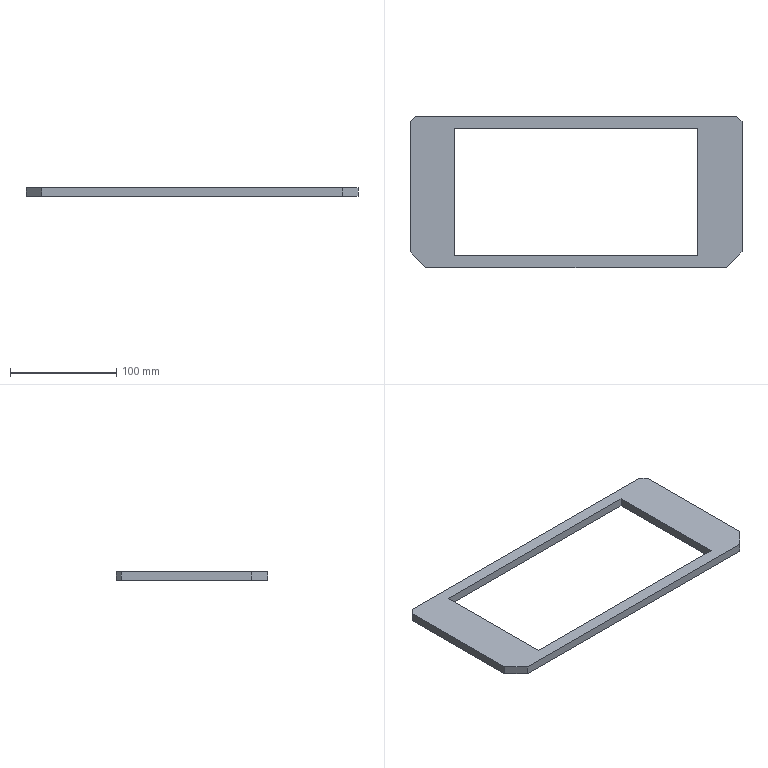Part | STEP file | A_SYL0380DJ1008_1_4-3_CHACHE_AS | 1 solid | 14 faces | box 313 x 143 x 8 mm | volume 135272 mm3 | plane 14
STEP:
#1=CARTESIAN_POINT('',(115.,-60.,8.));
#2=VERTEX_POINT('',#1);
#3=CARTESIAN_POINT('',(115.,-60.,0.));
#4=VERTEX_POINT('',#3);
#5=CARTESIAN_POINT('',(115.,-60.,8.));
#6=DIRECTION('',(0.,0.,-1.));
#7=VECTOR('',#6,1000.);
#8=LINE('',#5,#7);
#9=EDGE_CURVE('',#2,#4,#8,.T.);
#10=ORIENTED_EDGE('',*,*,#9,.T.);
#11=CARTESIAN_POINT('',(-115.,-60.,0.));
#12=VERTEX_POINT('',#11);
#13=CARTESIAN_POINT('',(-115.,-60.,0.));
#14=DIRECTION('',(1.,0.,0.));
#15=VECTOR('',#14,1000.);
#16=LINE('',#13,#15);
#17=EDGE_CURVE('',#12,#4,#16,.T.);
#18=ORIENTED_EDGE('',*,*,#17,.F.);
#19=CARTESIAN_POINT('',(-115.,-60.,8.));
#20=VERTEX_POINT('',#19);
#21=CARTESIAN_POINT('',(-115.,-60.,8.));
#22=DIRECTION('',(0.,0.,-1.));
#23=VECTOR('',#22,1000.);
#24=LINE('',#21,#23);
#25=EDGE_CURVE('',#20,#12,#24,.T.);
#26=ORIENTED_EDGE('',*,*,#25,.F.);
#27=CARTESIAN_POINT('',(-115.,-60.,8.));
#28=DIRECTION('',(1.,0.,0.));
#29=VECTOR('',#28,1000.);
#30=LINE('',#27,#29);
#31=EDGE_CURVE('',#20,#2,#30,.T.);
#32=ORIENTED_EDGE('',*,*,#31,.T.);
#33=EDGE_LOOP('',(#10,#18,#26,#32));
#34=FACE_OUTER_BOUND('',#33,.T.);
#35=CARTESIAN_POINT('',(0.,-60.,4.));
#36=DIRECTION('',(0.,-1.,0.));
#37=DIRECTION('',(0.,0.,-1.));
#38=AXIS2_PLACEMENT_3D('',#35,#36,#37);
#39=PLANE('',#38);
#40=ADVANCED_FACE('',(#34),#39,.F.);
#41=CARTESIAN_POINT('',(115.,60.,8.));
#42=VERTEX_POINT('',#41);
#43=CARTESIAN_POINT('',(115.,60.,0.));
#44=VERTEX_POINT('',#43);
#45=CARTESIAN_POINT('',(115.,60.,8.));
#46=DIRECTION('',(0.,0.,-1.));
#47=VECTOR('',#46,1000.);
#48=LINE('',#45,#47);
#49=EDGE_CURVE('',#42,#44,#48,.T.);
#50=ORIENTED_EDGE('',*,*,#49,.T.);
#51=CARTESIAN_POINT('',(115.,-60.,0.));
#52=DIRECTION('',(0.,1.,0.));
#53=VECTOR('',#52,1000.);
#54=LINE('',#51,#53);
#55=EDGE_CURVE('',#4,#44,#54,.T.);
#56=ORIENTED_EDGE('',*,*,#55,.F.);
#57=ORIENTED_EDGE('',*,*,#9,.F.);
#58=CARTESIAN_POINT('',(115.,-60.,8.));
#59=DIRECTION('',(0.,1.,0.));
#60=VECTOR('',#59,1000.);
#61=LINE('',#58,#60);
#62=EDGE_CURVE('',#2,#42,#61,.T.);
#63=ORIENTED_EDGE('',*,*,#62,.T.);
#64=EDGE_LOOP('',(#50,#56,#57,#63));
#65=FACE_OUTER_BOUND('',#64,.T.);
#66=CARTESIAN_POINT('',(115.,0.,4.));
#67=DIRECTION('',(1.,0.,0.));
#68=DIRECTION('',(0.,1.,0.));
#69=AXIS2_PLACEMENT_3D('',#66,#67,#68);
#70=PLANE('',#69);
#71=ADVANCED_FACE('',(#65),#70,.F.);
#72=CARTESIAN_POINT('',(-115.,60.,0.));
#73=VERTEX_POINT('',#72);
#74=CARTESIAN_POINT('',(-115.,60.,8.));
#75=VERTEX_POINT('',#74);
#76=CARTESIAN_POINT('',(-115.,60.,0.));
#77=DIRECTION('',(0.,0.,1.));
#78=VECTOR('',#77,1000.);
#79=LINE('',#76,#78);
#80=EDGE_CURVE('',#73,#75,#79,.T.);
#81=ORIENTED_EDGE('',*,*,#80,.F.);
#82=CARTESIAN_POINT('',(115.,60.,0.));
#83=DIRECTION('',(-1.,0.,0.));
#84=VECTOR('',#83,1000.);
#85=LINE('',#82,#84);
#86=EDGE_CURVE('',#44,#73,#85,.T.);
#87=ORIENTED_EDGE('',*,*,#86,.F.);
#88=ORIENTED_EDGE('',*,*,#49,.F.);
#89=CARTESIAN_POINT('',(115.,60.,8.));
#90=DIRECTION('',(-1.,0.,0.));
#91=VECTOR('',#90,1000.);
#92=LINE('',#89,#91);
#93=EDGE_CURVE('',#42,#75,#92,.T.);
#94=ORIENTED_EDGE('',*,*,#93,.T.);
#95=EDGE_LOOP('',(#81,#87,#88,#94));
#96=FACE_OUTER_BOUND('',#95,.T.);
#97=CARTESIAN_POINT('',(0.,60.,4.));
#98=DIRECTION('',(0.,1.,0.));
#99=DIRECTION('',(1.,0.,0.));
#100=AXIS2_PLACEMENT_3D('',#97,#98,#99);
#101=PLANE('',#100);
#102=ADVANCED_FACE('',(#96),#101,.F.);
#103=ORIENTED_EDGE('',*,*,#25,.T.);
#104=CARTESIAN_POINT('',(-115.,60.,0.));
#105=DIRECTION('',(0.,-1.,0.));
#106=VECTOR('',#105,1000.);
#107=LINE('',#104,#106);
#108=EDGE_CURVE('',#73,#12,#107,.T.);
#109=ORIENTED_EDGE('',*,*,#108,.F.);
#110=ORIENTED_EDGE('',*,*,#80,.T.);
#111=CARTESIAN_POINT('',(-115.,60.,8.));
#112=DIRECTION('',(0.,-1.,0.));
#113=VECTOR('',#112,1000.);
#114=LINE('',#111,#113);
#115=EDGE_CURVE('',#75,#20,#114,.T.);
#116=ORIENTED_EDGE('',*,*,#115,.T.);
#117=EDGE_LOOP('',(#103,#109,#110,#116));
#118=FACE_OUTER_BOUND('',#117,.T.);
#119=CARTESIAN_POINT('',(-115.,0.,4.));
#120=DIRECTION('',(-1.,0.,0.));
#121=DIRECTION('',(0.,0.,1.));
#122=AXIS2_PLACEMENT_3D('',#119,#120,#121);
#123=PLANE('',#122);
#124=ADVANCED_FACE('',(#118),#123,.F.);
#125=ORIENTED_EDGE('',*,*,#93,.F.);
#126=ORIENTED_EDGE('',*,*,#62,.F.);
#127=ORIENTED_EDGE('',*,*,#31,.F.);
#128=ORIENTED_EDGE('',*,*,#115,.F.);
#129=EDGE_LOOP('',(#125,#126,#127,#128));
#130=FACE_BOUND('',#129,.T.);
#131=CARTESIAN_POINT('',(-151.5,71.5,8.));
#132=VERTEX_POINT('',#131);
#133=CARTESIAN_POINT('',(-156.5,66.5,8.));
#134=VERTEX_POINT('',#133);
#135=CARTESIAN_POINT('',(-151.5,71.5,8.));
#136=DIRECTION('',(-0.7071,-0.7071,0.));
#137=VECTOR('',#136,1000.);
#138=LINE('',#135,#137);
#139=EDGE_CURVE('',#132,#134,#138,.T.);
#140=ORIENTED_EDGE('',*,*,#139,.T.);
#141=CARTESIAN_POINT('',(-156.5,-56.5,8.));
#142=VERTEX_POINT('',#141);
#143=CARTESIAN_POINT('',(-156.5,-56.5,8.));
#144=DIRECTION('',(0.,1.,0.));
#145=VECTOR('',#144,1000.);
#146=LINE('',#143,#145);
#147=EDGE_CURVE('',#142,#134,#146,.T.);
#148=ORIENTED_EDGE('',*,*,#147,.F.);
#149=CARTESIAN_POINT('',(-141.5,-71.5,8.));
#150=VERTEX_POINT('',#149);
#151=CARTESIAN_POINT('',(-156.5,-56.5,8.));
#152=DIRECTION('',(0.7071,-0.7071,0.));
#153=VECTOR('',#152,1000.);
#154=LINE('',#151,#153);
#155=EDGE_CURVE('',#142,#150,#154,.T.);
#156=ORIENTED_EDGE('',*,*,#155,.T.);
#157=CARTESIAN_POINT('',(141.5,-71.5,8.));
#158=VERTEX_POINT('',#157);
#159=CARTESIAN_POINT('',(141.5,-71.5,8.));
#160=DIRECTION('',(-1.,0.,0.));
#161=VECTOR('',#160,1000.);
#162=LINE('',#159,#161);
#163=EDGE_CURVE('',#158,#150,#162,.T.);
#164=ORIENTED_EDGE('',*,*,#163,.F.);
#165=CARTESIAN_POINT('',(156.5,-56.5,8.));
#166=VERTEX_POINT('',#165);
#167=CARTESIAN_POINT('',(141.5,-71.5,8.));
#168=DIRECTION('',(0.7071,0.7071,0.));
#169=VECTOR('',#168,1000.);
#170=LINE('',#167,#169);
#171=EDGE_CURVE('',#158,#166,#170,.T.);
#172=ORIENTED_EDGE('',*,*,#171,.T.);
#173=CARTESIAN_POINT('',(156.5,66.5,8.));
#174=VERTEX_POINT('',#173);
#175=CARTESIAN_POINT('',(156.5,66.5,8.));
#176=DIRECTION('',(0.,-1.,0.));
#177=VECTOR('',#176,1000.);
#178=LINE('',#175,#177);
#179=EDGE_CURVE('',#174,#166,#178,.T.);
#180=ORIENTED_EDGE('',*,*,#179,.F.);
#181=CARTESIAN_POINT('',(151.5,71.5,8.));
#182=VERTEX_POINT('',#181);
#183=CARTESIAN_POINT('',(156.5,66.5,8.));
#184=DIRECTION('',(-0.7071,0.7071,0.));
#185=VECTOR('',#184,1000.);
#186=LINE('',#183,#185);
#187=EDGE_CURVE('',#174,#182,#186,.T.);
#188=ORIENTED_EDGE('',*,*,#187,.T.);
#189=CARTESIAN_POINT('',(-151.5,71.5,8.));
#190=DIRECTION('',(1.,0.,0.));
#191=VECTOR('',#190,1000.);
#192=LINE('',#189,#191);
#193=EDGE_CURVE('',#132,#182,#192,.T.);
#194=ORIENTED_EDGE('',*,*,#193,.F.);
#195=EDGE_LOOP('',(#140,#148,#156,#164,#172,#180,#188,#194));
#196=FACE_OUTER_BOUND('',#195,.T.);
#197=CARTESIAN_POINT('',(0.,0.,8.));
#198=DIRECTION('',(0.,0.,1.));
#199=DIRECTION('',(1.,0.,0.));
#200=AXIS2_PLACEMENT_3D('',#197,#198,#199);
#201=PLANE('',#200);
#202=ADVANCED_FACE('',(#130,#196),#201,.T.);
#203=CARTESIAN_POINT('',(-151.5,71.5,0.));
#204=VERTEX_POINT('',#203);
#205=CARTESIAN_POINT('',(151.5,71.5,0.));
#206=VERTEX_POINT('',#205);
#207=CARTESIAN_POINT('',(-151.5,71.5,0.));
#208=DIRECTION('',(1.,0.,0.));
#209=VECTOR('',#208,1000.);
#210=LINE('',#207,#209);
#211=EDGE_CURVE('',#204,#206,#210,.T.);
#212=ORIENTED_EDGE('',*,*,#211,.F.);
#213=CARTESIAN_POINT('',(-151.5,71.5,0.));
#214=DIRECTION('',(0.,0.,1.));
#215=VECTOR('',#214,1000.);
#216=LINE('',#213,#215);
#217=EDGE_CURVE('',#204,#132,#216,.T.);
#218=ORIENTED_EDGE('',*,*,#217,.T.);
#219=ORIENTED_EDGE('',*,*,#193,.T.);
#220=CARTESIAN_POINT('',(151.5,71.5,8.));
#221=DIRECTION('',(0.,0.,-1.));
#222=VECTOR('',#221,1000.);
#223=LINE('',#220,#222);
#224=EDGE_CURVE('',#182,#206,#223,.T.);
#225=ORIENTED_EDGE('',*,*,#224,.T.);
#226=EDGE_LOOP('',(#212,#218,#219,#225));
#227=FACE_OUTER_BOUND('',#226,.T.);
#228=CARTESIAN_POINT('',(0.,71.5,4.));
#229=DIRECTION('',(0.,-1.,0.));
#230=DIRECTION('',(0.,0.,-1.));
#231=AXIS2_PLACEMENT_3D('',#228,#229,#230);
#232=PLANE('',#231);
#233=ADVANCED_FACE('',(#227),#232,.F.);
#234=CARTESIAN_POINT('',(-156.5,66.5,0.));
#235=VERTEX_POINT('',#234);
#236=CARTESIAN_POINT('',(-156.5,66.5,0.));
#237=DIRECTION('',(0.7071,0.7071,0.));
#238=VECTOR('',#237,1000.);
#239=LINE('',#236,#238);
#240=EDGE_CURVE('',#235,#204,#239,.T.);
#241=ORIENTED_EDGE('',*,*,#240,.F.);
#242=CARTESIAN_POINT('',(-156.5,66.5,8.));
#243=DIRECTION('',(0.,0.,-1.));
#244=VECTOR('',#243,1000.);
#245=LINE('',#242,#244);
#246=EDGE_CURVE('',#134,#235,#245,.T.);
#247=ORIENTED_EDGE('',*,*,#246,.F.);
#248=ORIENTED_EDGE('',*,*,#139,.F.);
#249=ORIENTED_EDGE('',*,*,#217,.F.);
#250=EDGE_LOOP('',(#241,#247,#248,#249));
#251=FACE_OUTER_BOUND('',#250,.T.);
#252=CARTESIAN_POINT('',(-154.,69.,4.));
#253=DIRECTION('',(-0.7071,0.7071,0.));
#254=DIRECTION('',(0.,0.,1.));
#255=AXIS2_PLACEMENT_3D('',#252,#253,#254);
#256=PLANE('',#255);
#257=ADVANCED_FACE('',(#251),#256,.T.);
#258=ORIENTED_EDGE('',*,*,#147,.T.);
#259=ORIENTED_EDGE('',*,*,#246,.T.);
#260=CARTESIAN_POINT('',(-156.5,-56.5,0.));
#261=VERTEX_POINT('',#260);
#262=CARTESIAN_POINT('',(-156.5,-56.5,0.));
#263=DIRECTION('',(0.,1.,0.));
#264=VECTOR('',#263,1000.);
#265=LINE('',#262,#264);
#266=EDGE_CURVE('',#261,#235,#265,.T.);
#267=ORIENTED_EDGE('',*,*,#266,.F.);
#268=CARTESIAN_POINT('',(-156.5,-56.5,0.));
#269=DIRECTION('',(0.,0.,1.));
#270=VECTOR('',#269,1000.);
#271=LINE('',#268,#270);
#272=EDGE_CURVE('',#261,#142,#271,.T.);
#273=ORIENTED_EDGE('',*,*,#272,.T.);
#274=EDGE_LOOP('',(#258,#259,#267,#273));
#275=FACE_OUTER_BOUND('',#274,.T.);
#276=CARTESIAN_POINT('',(-156.5,0.,4.));
#277=DIRECTION('',(1.,0.,0.));
#278=DIRECTION('',(0.,1.,0.));
#279=AXIS2_PLACEMENT_3D('',#276,#277,#278);
#280=PLANE('',#279);
#281=ADVANCED_FACE('',(#275),#280,.F.);
#282=CARTESIAN_POINT('',(-141.5,-71.5,0.));
#283=VERTEX_POINT('',#282);
#284=CARTESIAN_POINT('',(-141.5,-71.5,0.));
#285=DIRECTION('',(-0.7071,0.7071,0.));
#286=VECTOR('',#285,1000.);
#287=LINE('',#284,#286);
#288=EDGE_CURVE('',#283,#261,#287,.T.);
#289=ORIENTED_EDGE('',*,*,#288,.F.);
#290=CARTESIAN_POINT('',(-141.5,-71.5,8.));
#291=DIRECTION('',(0.,0.,-1.));
#292=VECTOR('',#291,1000.);
#293=LINE('',#290,#292);
#294=EDGE_CURVE('',#150,#283,#293,.T.);
#295=ORIENTED_EDGE('',*,*,#294,.F.);
#296=ORIENTED_EDGE('',*,*,#155,.F.);
#297=ORIENTED_EDGE('',*,*,#272,.F.);
#298=EDGE_LOOP('',(#289,#295,#296,#297));
#299=FACE_OUTER_BOUND('',#298,.T.);
#300=CARTESIAN_POINT('',(-149.,-64.,4.));
#301=DIRECTION('',(-0.7071,-0.7071,0.));
#302=DIRECTION('',(-0.7071,0.7071,0.));
#303=AXIS2_PLACEMENT_3D('',#300,#301,#302);
#304=PLANE('',#303);
#305=ADVANCED_FACE('',(#299),#304,.T.);
#306=ORIENTED_EDGE('',*,*,#163,.T.);
#307=ORIENTED_EDGE('',*,*,#294,.T.);
#308=CARTESIAN_POINT('',(141.5,-71.5,0.));
#309=VERTEX_POINT('',#308);
#310=CARTESIAN_POINT('',(141.5,-71.5,0.));
#311=DIRECTION('',(-1.,0.,0.));
#312=VECTOR('',#311,1000.);
#313=LINE('',#310,#312);
#314=EDGE_CURVE('',#309,#283,#313,.T.);
#315=ORIENTED_EDGE('',*,*,#314,.F.);
#316=CARTESIAN_POINT('',(141.5,-71.5,0.));
#317=DIRECTION('',(0.,0.,1.));
#318=VECTOR('',#317,1000.);
#319=LINE('',#316,#318);
#320=EDGE_CURVE('',#309,#158,#319,.T.);
#321=ORIENTED_EDGE('',*,*,#320,.T.);
#322=EDGE_LOOP('',(#306,#307,#315,#321));
#323=FACE_OUTER_BOUND('',#322,.T.);
#324=CARTESIAN_POINT('',(0.,-71.5,4.));
#325=DIRECTION('',(0.,1.,0.));
#326=DIRECTION('',(1.,0.,0.));
#327=AXIS2_PLACEMENT_3D('',#324,#325,#326);
#328=PLANE('',#327);
#329=ADVANCED_FACE('',(#323),#328,.F.);
#330=CARTESIAN_POINT('',(156.5,-56.5,0.));
#331=VERTEX_POINT('',#330);
#332=CARTESIAN_POINT('',(156.5,-56.5,0.));
#333=DIRECTION('',(-0.7071,-0.7071,0.));
#334=VECTOR('',#333,1000.);
#335=LINE('',#332,#334);
#336=EDGE_CURVE('',#331,#309,#335,.T.);
#337=ORIENTED_EDGE('',*,*,#336,.F.);
#338=CARTESIAN_POINT('',(156.5,-56.5,8.));
#339=DIRECTION('',(0.,0.,-1.));
#340=VECTOR('',#339,1000.);
#341=LINE('',#338,#340);
#342=EDGE_CURVE('',#166,#331,#341,.T.);
#343=ORIENTED_EDGE('',*,*,#342,.F.);
#344=ORIENTED_EDGE('',*,*,#171,.F.);
#345=ORIENTED_EDGE('',*,*,#320,.F.);
#346=EDGE_LOOP('',(#337,#343,#344,#345));
#347=FACE_OUTER_BOUND('',#346,.T.);
#348=CARTESIAN_POINT('',(149.,-64.,4.));
#349=DIRECTION('',(0.7071,-0.7071,0.));
#350=DIRECTION('',(0.,0.,-1.));
#351=AXIS2_PLACEMENT_3D('',#348,#349,#350);
#352=PLANE('',#351);
#353=ADVANCED_FACE('',(#347),#352,.T.);
#354=CARTESIAN_POINT('',(156.5,66.5,0.));
#355=VERTEX_POINT('',#354);
#356=CARTESIAN_POINT('',(156.5,66.5,0.));
#357=DIRECTION('',(0.,-1.,0.));
#358=VECTOR('',#357,1000.);
#359=LINE('',#356,#358);
#360=EDGE_CURVE('',#355,#331,#359,.T.);
#361=ORIENTED_EDGE('',*,*,#360,.F.);
#362=CARTESIAN_POINT('',(156.5,66.5,0.));
#363=DIRECTION('',(0.,0.,1.));
#364=VECTOR('',#363,1000.);
#365=LINE('',#362,#364);
#366=EDGE_CURVE('',#355,#174,#365,.T.);
#367=ORIENTED_EDGE('',*,*,#366,.T.);
#368=ORIENTED_EDGE('',*,*,#179,.T.);
#369=ORIENTED_EDGE('',*,*,#342,.T.);
#370=EDGE_LOOP('',(#361,#367,#368,#369));
#371=FACE_OUTER_BOUND('',#370,.T.);
#372=CARTESIAN_POINT('',(156.5,0.,4.));
#373=DIRECTION('',(-1.,0.,0.));
#374=DIRECTION('',(0.,0.,1.));
#375=AXIS2_PLACEMENT_3D('',#372,#373,#374);
#376=PLANE('',#375);
#377=ADVANCED_FACE('',(#371),#376,.F.);
#378=CARTESIAN_POINT('',(151.5,71.5,0.));
#379=DIRECTION('',(0.7071,-0.7071,0.));
#380=VECTOR('',#379,1000.);
#381=LINE('',#378,#380);
#382=EDGE_CURVE('',#206,#355,#381,.T.);
#383=ORIENTED_EDGE('',*,*,#382,.F.);
#384=ORIENTED_EDGE('',*,*,#224,.F.);
#385=ORIENTED_EDGE('',*,*,#187,.F.);
#386=ORIENTED_EDGE('',*,*,#366,.F.);
#387=EDGE_LOOP('',(#383,#384,#385,#386));
#388=FACE_OUTER_BOUND('',#387,.T.);
#389=CARTESIAN_POINT('',(154.,69.,4.));
#390=DIRECTION('',(0.7071,0.7071,0.));
#391=DIRECTION('',(0.,0.,-1.));
#392=AXIS2_PLACEMENT_3D('',#389,#390,#391);
#393=PLANE('',#392);
#394=ADVANCED_FACE('',(#388),#393,.T.);
#395=ORIENTED_EDGE('',*,*,#55,.T.);
#396=ORIENTED_EDGE('',*,*,#86,.T.);
#397=ORIENTED_EDGE('',*,*,#108,.T.);
#398=ORIENTED_EDGE('',*,*,#17,.T.);
#399=EDGE_LOOP('',(#395,#396,#397,#398));
#400=FACE_BOUND('',#399,.T.);
#401=ORIENTED_EDGE('',*,*,#360,.T.);
#402=ORIENTED_EDGE('',*,*,#336,.T.);
#403=ORIENTED_EDGE('',*,*,#314,.T.);
#404=ORIENTED_EDGE('',*,*,#288,.T.);
#405=ORIENTED_EDGE('',*,*,#266,.T.);
#406=ORIENTED_EDGE('',*,*,#240,.T.);
#407=ORIENTED_EDGE('',*,*,#211,.T.);
#408=ORIENTED_EDGE('',*,*,#382,.T.);
#409=EDGE_LOOP('',(#401,#402,#403,#404,#405,#406,#407,#408));
#410=FACE_OUTER_BOUND('',#409,.T.);
#411=CARTESIAN_POINT('',(0.,0.,0.));
#412=DIRECTION('',(0.,0.,1.));
#413=DIRECTION('',(1.,0.,0.));
#414=AXIS2_PLACEMENT_3D('',#411,#412,#413);
#415=PLANE('',#414);
#416=ADVANCED_FACE('',(#400,#410),#415,.F.);
#417=CLOSED_SHELL('',(#40,#71,#102,#124,#202,#233,#257,#281,#305,#329,#353,#377,#394,#416));
#418=MANIFOLD_SOLID_BREP('',#417);
#419=CARTESIAN_POINT('',(0.,0.,0.));
#420=DIRECTION('',(0.,0.,1.));
#421=DIRECTION('',(1.,0.,0.));
#422=AXIS2_PLACEMENT_3D('',#419,#420,#421);
#423=(LENGTH_UNIT()NAMED_UNIT(*)SI_UNIT(.MILLI.,.METRE.));
#424=UNCERTAINTY_MEASURE_WITH_UNIT(LENGTH_MEASURE(0.00001),#423,'','');
#425=(NAMED_UNIT(*)PLANE_ANGLE_UNIT()SI_UNIT($,.RADIAN.));
#426=(NAMED_UNIT(*)SI_UNIT($,.STERADIAN.)SOLID_ANGLE_UNIT());
#427=(GEOMETRIC_REPRESENTATION_CONTEXT(3)GLOBAL_UNCERTAINTY_ASSIGNED_CONTEXT((#424))GLOBAL_UNIT_ASSIGNED_CONTEXT((#423,#425,#426))REPRESENTATION_CONTEXT('',''));
#428=ADVANCED_BREP_SHAPE_REPRESENTATION('',(#418,#422),#427);